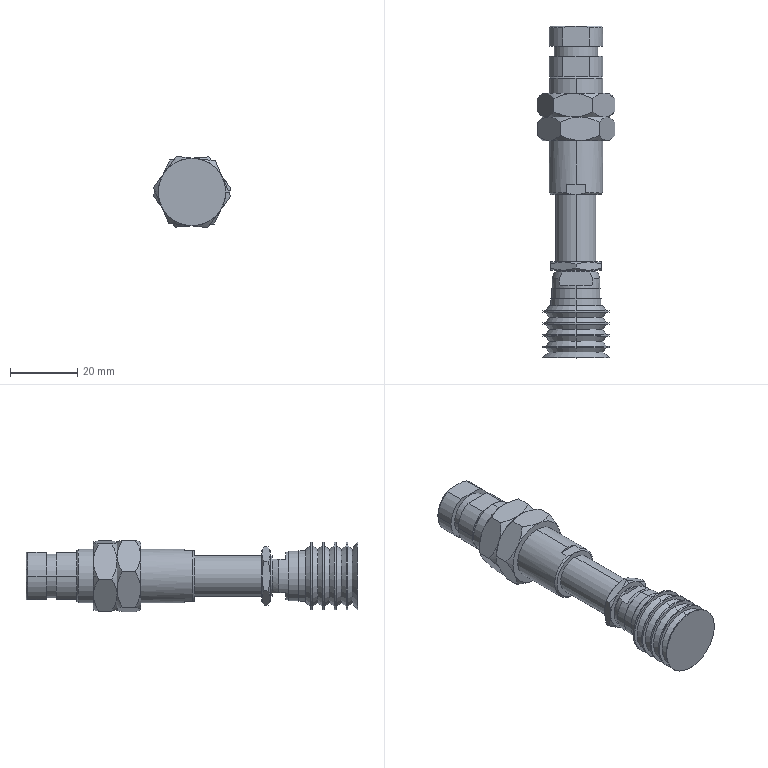Part | STEP file | vacuum suction cup assembly 4.5-fold bellows type standard type GXSE[GXSE-d20-20] | 1 solid | 166 faces | box 23.018 x 98.5 x 21.189 mm | volume 17845 mm3 | cone 69 | plane 61 | cylinder 36 | commonest cylinder face diameters 16 x10 20 x10 8.556 x4 12 x4 13 x2 14.2 x2